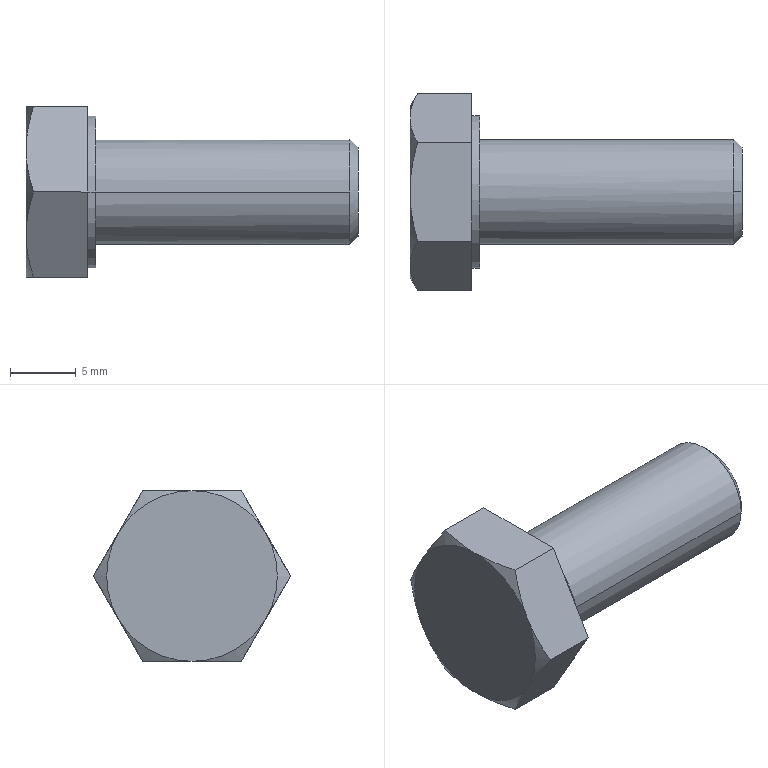Part | STEP file | 1 solid | 22 faces | box 25.3 x 15.011 x 13 mm | volume 1750 mm3 | plane 10 | cone 8 | cylinder 4 | commonest cylinder face diameters 8 x2 11.63 x2